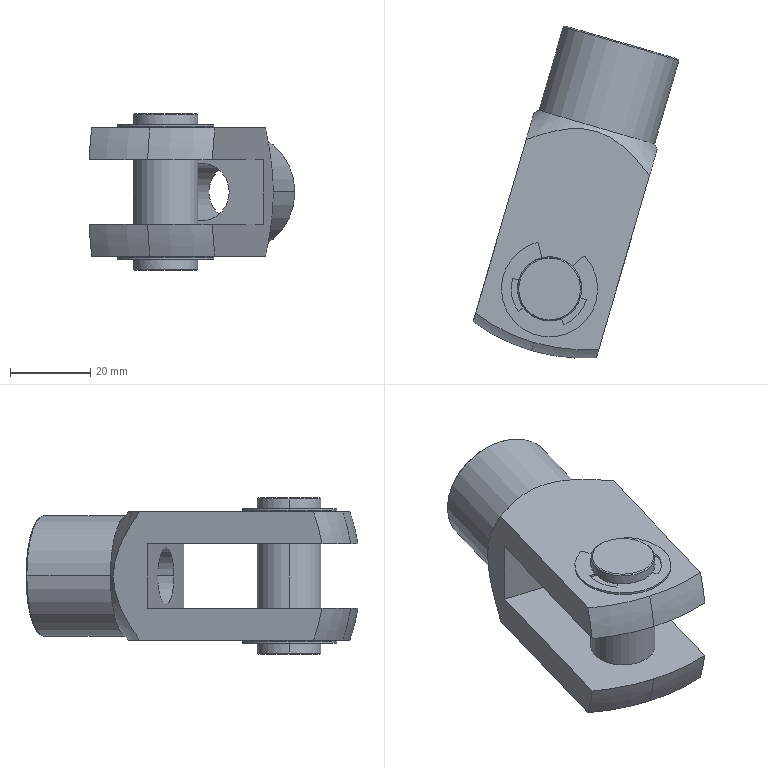Part | SolidWorks | features BaseBody 1 | 1 solid | 75 faces | box 51.292 x 82.808 x 39 mm | volume 48232 mm3 | plane 32 | cylinder 29 | cone 10 | spline 4 | commonest cylinder face diameters 16 x6 24 x6 19.2 x5 1 x4 14.4 x4 14.376 x2